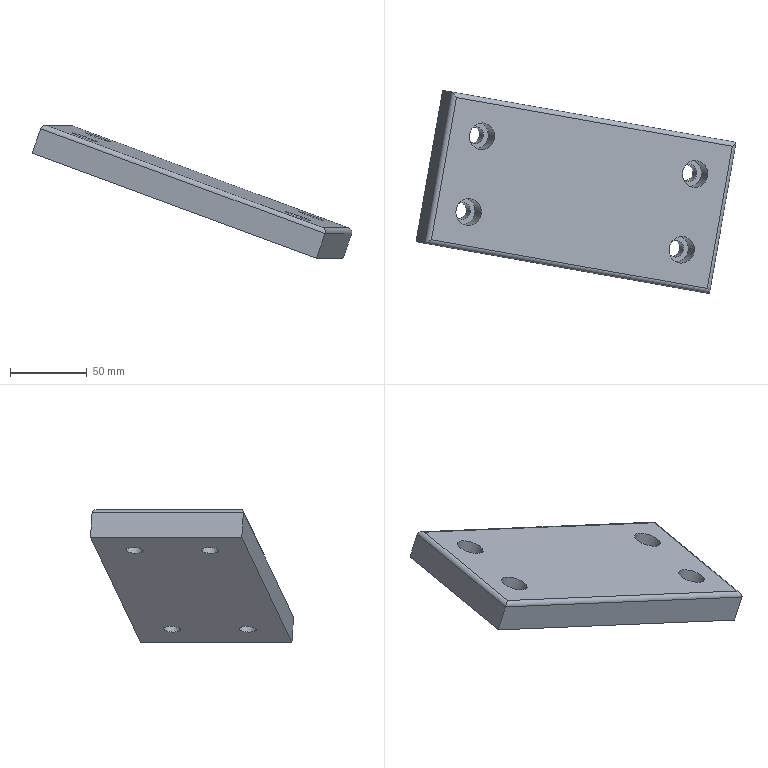Part | NX | features solid 2 | 1 solid | 22 faces | box 208.326 x 132.13 x 86.353 mm | volume 384265 mm3 | cylinder 12 | plane 10 | commonest cylinder face diameters 6 x4 11 x4 17.5 x4
STEP:
#1=CARTESIAN_POINT('',(-905.367,162.289,-231.832));
#2=VERTEX_POINT('',#1);
#3=CARTESIAN_POINT('',(-1090.45,194.924,-163.428));
#4=VERTEX_POINT('',#3);
#5=CARTESIAN_POINT('',(-905.275,162.273,-231.866));
#6=DIRECTION('',(-0.9254,0.1632,0.342));
#7=VECTOR('',#6,1000.);
#8=LINE('',#5,#7);
#9=EDGE_CURVE('',#2,#4,#8,.T.);
#10=ORIENTED_EDGE('',*,*,#9,.T.);
#11=CARTESIAN_POINT('',(-1096.176,195.934,-179.402));
#12=VERTEX_POINT('',#11);
#13=CARTESIAN_POINT('',(-1089.406,194.74,-160.515));
#14=DIRECTION('',(-0.3368,0.05939,-0.9397));
#15=VECTOR('',#14,1000.);
#16=LINE('',#13,#15);
#17=EDGE_CURVE('',#4,#12,#16,.T.);
#18=ORIENTED_EDGE('',*,*,#17,.T.);
#19=CARTESIAN_POINT('',(-911.093,163.299,-247.806));
#20=VERTEX_POINT('',#19);
#21=CARTESIAN_POINT('',(-910.908,163.266,-247.875));
#22=DIRECTION('',(-0.9254,0.1632,0.342));
#23=VECTOR('',#22,1000.);
#24=LINE('',#21,#23);
#25=EDGE_CURVE('',#20,#12,#24,.T.);
#26=ORIENTED_EDGE('',*,*,#25,.F.);
#27=CARTESIAN_POINT('',(-911.464,163.364,-248.84));
#28=DIRECTION('',(0.3368,-0.05939,0.9397));
#29=VECTOR('',#28,1000.);
#30=LINE('',#27,#29);
#31=EDGE_CURVE('',#2,#20,#30,.F.);
#32=ORIENTED_EDGE('',*,*,#31,.F.);
#33=EDGE_LOOP('',(#10,#18,#26,#32));
#34=FACE_BOUND('',#33,.T.);
#35=CARTESIAN_POINT('',(-904.23,162.089,-228.953));
#36=DIRECTION('',(-0.1736,-0.9848,0.));
#37=DIRECTION('',(-0.9254,0.1632,0.342));
#38=AXIS2_PLACEMENT_3D('',#35,#36,#37);
#39=PLANE('',#38);
#40=ADVANCED_FACE('',(#34),#39,.T.);
#41=CARTESIAN_POINT('',(-906.612,165.555,-227.987));
#42=VERTEX_POINT('',#41);
#43=CARTESIAN_POINT('',(-907.622,165.733,-230.806));
#44=DIRECTION('',(0.7772,0.581,-0.2418));
#45=DIRECTION('',(-0.5316,0.8117,0.2418));
#46=AXIS2_PLACEMENT_3D('',#43,#44,#45);
#47=ELLIPSE('',#46,4.243,3.);
#48=EDGE_CURVE('',#42,#2,#47,.T.);
#49=ORIENTED_EDGE('',*,*,#48,.T.);
#50=CARTESIAN_POINT('',(-888.002,260.77,-231.832));
#51=VERTEX_POINT('',#50);
#52=CARTESIAN_POINT('',(-906.053,158.399,-231.832));
#53=DIRECTION('',(0.1736,0.9848,0.));
#54=VECTOR('',#53,1000.);
#55=LINE('',#52,#54);
#56=EDGE_CURVE('',#51,#2,#55,.F.);
#57=ORIENTED_EDGE('',*,*,#56,.F.);
#58=CARTESIAN_POINT('',(-890.289,258.127,-227.987));
#59=VERTEX_POINT('',#58);
#60=CARTESIAN_POINT('',(-891.3,258.305,-230.806));
#61=DIRECTION('',(-0.5316,0.8117,0.2418));
#62=DIRECTION('',(0.7772,0.581,-0.2418));
#63=AXIS2_PLACEMENT_3D('',#60,#61,#62);
#64=ELLIPSE('',#63,4.243,3.);
#65=EDGE_CURVE('',#59,#51,#64,.T.);
#66=ORIENTED_EDGE('',*,*,#65,.F.);
#67=CARTESIAN_POINT('',(-887.58,273.49,-227.987));
#68=DIRECTION('',(0.1736,0.9848,0.));
#69=VECTOR('',#68,1000.);
#70=LINE('',#67,#69);
#71=EDGE_CURVE('',#42,#59,#70,.T.);
#72=ORIENTED_EDGE('',*,*,#71,.F.);
#73=EDGE_LOOP('',(#49,#57,#66,#72));
#74=FACE_BOUND('',#73,.T.);
#75=CARTESIAN_POINT('',(-888.591,273.668,-230.806));
#76=DIRECTION('',(0.1736,0.9848,0.));
#77=DIRECTION('',(-0.9848,0.1736,0.));
#78=AXIS2_PLACEMENT_3D('',#75,#76,#77);
#79=CYLINDRICAL_SURFACE('',#78,3.);
#80=ADVANCED_FACE('',(#74),#79,.T.);
#81=CARTESIAN_POINT('',(-1086.143,197.211,-161.635));
#82=VERTEX_POINT('',#81);
#83=CARTESIAN_POINT('',(-903.651,165.033,-229.081));
#84=DIRECTION('',(-0.9254,0.1632,0.342));
#85=VECTOR('',#84,1000.);
#86=LINE('',#83,#85);
#87=EDGE_CURVE('',#82,#42,#86,.F.);
#88=ORIENTED_EDGE('',*,*,#87,.F.);
#89=CARTESIAN_POINT('',(-1087.153,197.389,-164.454));
#90=DIRECTION('',(-0.5316,0.8117,0.2418));
#91=DIRECTION('',(-0.7772,-0.581,0.2418));
#92=AXIS2_PLACEMENT_3D('',#89,#90,#91);
#93=ELLIPSE('',#92,4.243,3.);
#94=EDGE_CURVE('',#4,#82,#93,.T.);
#95=ORIENTED_EDGE('',*,*,#94,.F.);
#96=ORIENTED_EDGE('',*,*,#9,.F.);
#97=ORIENTED_EDGE('',*,*,#48,.F.);
#98=EDGE_LOOP('',(#88,#95,#96,#97));
#99=FACE_BOUND('',#98,.T.);
#100=CARTESIAN_POINT('',(-904.754,165.227,-231.866));
#101=DIRECTION('',(-0.9254,0.1632,0.342));
#102=DIRECTION('',(0.3368,-0.05939,0.9397));
#103=AXIS2_PLACEMENT_3D('',#100,#101,#102);
#104=CYLINDRICAL_SURFACE('',#103,3.);
#105=ADVANCED_FACE('',(#99),#104,.T.);
#106=ORIENTED_EDGE('',*,*,#71,.T.);
#107=CARTESIAN_POINT('',(-1069.82,289.783,-161.635));
#108=VERTEX_POINT('',#107);
#109=CARTESIAN_POINT('',(-887.328,257.605,-229.081));
#110=DIRECTION('',(-0.9254,0.1632,0.342));
#111=VECTOR('',#110,1000.);
#112=LINE('',#109,#111);
#113=EDGE_CURVE('',#59,#108,#112,.T.);
#114=ORIENTED_EDGE('',*,*,#113,.T.);
#115=CARTESIAN_POINT('',(-1067.111,305.146,-161.635));
#116=DIRECTION('',(0.1736,0.9848,0.));
#117=VECTOR('',#116,1000.);
#118=LINE('',#115,#117);
#119=EDGE_CURVE('',#108,#82,#118,.F.);
#120=ORIENTED_EDGE('',*,*,#119,.T.);
#121=ORIENTED_EDGE('',*,*,#87,.T.);
#122=EDGE_LOOP('',(#106,#114,#120,#121));
#123=FACE_BOUND('',#122,.T.);
#124=CARTESIAN_POINT('',(-922.566,241.479,-217.469));
#125=VERTEX_POINT('',#124);
#126=CARTESIAN_POINT('',(-914.468,240.051,-220.462));
#127=DIRECTION('',(-0.3368,0.05939,-0.9397));
#128=DIRECTION('',(-0.9254,0.1632,0.342));
#129=AXIS2_PLACEMENT_3D('',#126,#127,#128);
#130=CIRCLE('',#129,8.75);
#131=EDGE_CURVE('',#125,#125,#130,.T.);
#132=ORIENTED_EDGE('',*,*,#131,.T.);
#133=EDGE_LOOP('',(#132));
#134=FACE_BOUND('',#133,.T.);
#135=CARTESIAN_POINT('',(-931.248,192.238,-217.469));
#136=VERTEX_POINT('',#135);
#137=CARTESIAN_POINT('',(-923.151,190.811,-220.462));
#138=DIRECTION('',(-0.3368,0.05939,-0.9397));
#139=DIRECTION('',(-0.9254,0.1632,0.342));
#140=AXIS2_PLACEMENT_3D('',#137,#138,#139);
#141=CIRCLE('',#140,8.75);
#142=EDGE_CURVE('',#136,#136,#141,.T.);
#143=ORIENTED_EDGE('',*,*,#142,.T.);
#144=EDGE_LOOP('',(#143));
#145=FACE_BOUND('',#144,.T.);
#146=CARTESIAN_POINT('',(-1053.866,213.859,-172.152));
#147=VERTEX_POINT('',#146);
#148=CARTESIAN_POINT('',(-1061.963,215.287,-169.159));
#149=DIRECTION('',(0.3368,-0.05939,0.9397));
#150=DIRECTION('',(0.9254,-0.1632,-0.342));
#151=AXIS2_PLACEMENT_3D('',#148,#149,#150);
#152=CIRCLE('',#151,8.75);
#153=EDGE_CURVE('',#147,#147,#152,.F.);
#154=ORIENTED_EDGE('',*,*,#153,.T.);
#155=EDGE_LOOP('',(#154));
#156=FACE_BOUND('',#155,.T.);
#157=CARTESIAN_POINT('',(-1045.184,263.1,-172.152));
#158=VERTEX_POINT('',#157);
#159=CARTESIAN_POINT('',(-1053.281,264.527,-169.159));
#160=DIRECTION('',(0.3368,-0.05939,0.9397));
#161=DIRECTION('',(0.9254,-0.1632,-0.342));
#162=AXIS2_PLACEMENT_3D('',#159,#160,#161);
#163=CIRCLE('',#162,8.75);
#164=EDGE_CURVE('',#158,#158,#163,.F.);
#165=ORIENTED_EDGE('',*,*,#164,.T.);
#166=EDGE_LOOP('',(#165));
#167=FACE_BOUND('',#166,.T.);
#168=CARTESIAN_POINT('',(-884.619,272.968,-229.081));
#169=DIRECTION('',(0.3368,-0.05939,0.9397));
#170=DIRECTION('',(-0.9254,0.1632,0.342));
#171=AXIS2_PLACEMENT_3D('',#168,#169,#170);
#172=PLANE('',#171);
#173=ADVANCED_FACE('',(#123,#134,#145,#156,#167),#172,.T.);
#174=ORIENTED_EDGE('',*,*,#31,.T.);
#175=CARTESIAN_POINT('',(-893.728,261.78,-247.806));
#176=VERTEX_POINT('',#175);
#177=CARTESIAN_POINT('',(-891.558,274.09,-247.806));
#178=DIRECTION('',(-0.1736,-0.9848,0.));
#179=VECTOR('',#178,1000.);
#180=LINE('',#177,#179);
#181=EDGE_CURVE('',#176,#20,#180,.T.);
#182=ORIENTED_EDGE('',*,*,#181,.F.);
#183=CARTESIAN_POINT('',(-894.099,261.845,-248.84));
#184=DIRECTION('',(0.3368,-0.05939,0.9397));
#185=VECTOR('',#184,1000.);
#186=LINE('',#183,#185);
#187=EDGE_CURVE('',#176,#51,#186,.T.);
#188=ORIENTED_EDGE('',*,*,#187,.T.);
#189=ORIENTED_EDGE('',*,*,#56,.T.);
#190=EDGE_LOOP('',(#174,#182,#188,#189));
#191=FACE_BOUND('',#190,.T.);
#192=CARTESIAN_POINT('',(-912.15,159.474,-248.84));
#193=DIRECTION('',(0.9254,-0.1632,-0.342));
#194=DIRECTION('',(0.1736,0.9848,0.));
#195=AXIS2_PLACEMENT_3D('',#192,#193,#194);
#196=PLANE('',#195);
#197=ADVANCED_FACE('',(#191),#196,.T.);
#198=ORIENTED_EDGE('',*,*,#25,.T.);
#199=CARTESIAN_POINT('',(-1078.812,294.415,-179.402));
#200=VERTEX_POINT('',#199);
#201=CARTESIAN_POINT('',(-1093.85,209.13,-179.402));
#202=DIRECTION('',(-0.1736,-0.9848,0.));
#203=VECTOR('',#202,1000.);
#204=LINE('',#201,#203);
#205=EDGE_CURVE('',#200,#12,#204,.T.);
#206=ORIENTED_EDGE('',*,*,#205,.F.);
#207=CARTESIAN_POINT('',(-893.543,261.747,-247.875));
#208=DIRECTION('',(0.9254,-0.1632,-0.342));
#209=VECTOR('',#208,1000.);
#210=LINE('',#207,#209);
#211=EDGE_CURVE('',#200,#176,#210,.T.);
#212=ORIENTED_EDGE('',*,*,#211,.T.);
#213=ORIENTED_EDGE('',*,*,#181,.T.);
#214=EDGE_LOOP('',(#198,#206,#212,#213));
#215=FACE_BOUND('',#214,.T.);
#216=CARTESIAN_POINT('',(-926.295,242.136,-237.375));
#217=VERTEX_POINT('',#216);
#218=CARTESIAN_POINT('',(-921.205,241.239,-239.256));
#219=DIRECTION('',(-0.3368,0.05939,-0.9397));
#220=DIRECTION('',(-0.9254,0.1632,0.342));
#221=AXIS2_PLACEMENT_3D('',#218,#219,#220);
#222=CIRCLE('',#221,5.5);
#223=EDGE_CURVE('',#217,#217,#222,.T.);
#224=ORIENTED_EDGE('',*,*,#223,.F.);
#225=EDGE_LOOP('',(#224));
#226=FACE_BOUND('',#225,.T.);
#227=CARTESIAN_POINT('',(-934.977,192.896,-237.375));
#228=VERTEX_POINT('',#227);
#229=CARTESIAN_POINT('',(-929.887,191.998,-239.256));
#230=DIRECTION('',(-0.3368,0.05939,-0.9397));
#231=DIRECTION('',(-0.9254,0.1632,0.342));
#232=AXIS2_PLACEMENT_3D('',#229,#230,#231);
#233=CIRCLE('',#232,5.5);
#234=EDGE_CURVE('',#228,#228,#233,.T.);
#235=ORIENTED_EDGE('',*,*,#234,.F.);
#236=EDGE_LOOP('',(#235));
#237=FACE_BOUND('',#236,.T.);
#238=CARTESIAN_POINT('',(-1073.79,217.372,-186.072));
#239=VERTEX_POINT('',#238);
#240=CARTESIAN_POINT('',(-1068.7,216.475,-187.953));
#241=DIRECTION('',(-0.3368,0.05939,-0.9397));
#242=DIRECTION('',(-0.9254,0.1632,0.342));
#243=AXIS2_PLACEMENT_3D('',#240,#241,#242);
#244=CIRCLE('',#243,5.5);
#245=EDGE_CURVE('',#239,#239,#244,.T.);
#246=ORIENTED_EDGE('',*,*,#245,.F.);
#247=EDGE_LOOP('',(#246));
#248=FACE_BOUND('',#247,.T.);
#249=CARTESIAN_POINT('',(-1065.107,266.613,-186.072));
#250=VERTEX_POINT('',#249);
#251=CARTESIAN_POINT('',(-1060.017,265.715,-187.953));
#252=DIRECTION('',(-0.3368,0.05939,-0.9397));
#253=DIRECTION('',(-0.9254,0.1632,0.342));
#254=AXIS2_PLACEMENT_3D('',#251,#252,#253);
#255=CIRCLE('',#254,5.5);
#256=EDGE_CURVE('',#250,#250,#255,.T.);
#257=ORIENTED_EDGE('',*,*,#256,.F.);
#258=EDGE_LOOP('',(#257));
#259=FACE_BOUND('',#258,.T.);
#260=CARTESIAN_POINT('',(-911.611,159.278,-247.875));
#261=DIRECTION('',(-0.3368,0.05939,-0.9397));
#262=DIRECTION('',(-0.9254,0.1632,0.342));
#263=AXIS2_PLACEMENT_3D('',#260,#261,#262);
#264=PLANE('',#263);
#265=ADVANCED_FACE('',(#215,#226,#237,#248,#259),#264,.T.);
#266=ORIENTED_EDGE('',*,*,#17,.F.);
#267=CARTESIAN_POINT('',(-1073.086,293.405,-163.428));
#268=VERTEX_POINT('',#267);
#269=CARTESIAN_POINT('',(-1088.124,208.121,-163.428));
#270=DIRECTION('',(0.1736,0.9848,0.));
#271=VECTOR('',#270,1000.);
#272=LINE('',#269,#271);
#273=EDGE_CURVE('',#4,#268,#272,.T.);
#274=ORIENTED_EDGE('',*,*,#273,.T.);
#275=CARTESIAN_POINT('',(-1072.041,293.221,-160.515));
#276=DIRECTION('',(-0.3368,0.05939,-0.9397));
#277=VECTOR('',#276,1000.);
#278=LINE('',#275,#277);
#279=EDGE_CURVE('',#268,#200,#278,.T.);
#280=ORIENTED_EDGE('',*,*,#279,.T.);
#281=ORIENTED_EDGE('',*,*,#205,.T.);
#282=EDGE_LOOP('',(#266,#274,#280,#281));
#283=FACE_BOUND('',#282,.T.);
#284=CARTESIAN_POINT('',(-1087.079,207.937,-160.515));
#285=DIRECTION('',(-0.9254,0.1632,0.342));
#286=DIRECTION('',(0.1736,0.9848,0.));
#287=AXIS2_PLACEMENT_3D('',#284,#285,#286);
#288=PLANE('',#287);
#289=ADVANCED_FACE('',(#283),#288,.T.);
#290=ORIENTED_EDGE('',*,*,#279,.F.);
#291=CARTESIAN_POINT('',(-881.062,259.546,-234.397));
#292=DIRECTION('',(-0.9254,0.1632,0.342));
#293=VECTOR('',#292,1000.);
#294=LINE('',#291,#293);
#295=EDGE_CURVE('',#268,#51,#294,.F.);
#296=ORIENTED_EDGE('',*,*,#295,.T.);
#297=ORIENTED_EDGE('',*,*,#187,.F.);
#298=ORIENTED_EDGE('',*,*,#211,.F.);
#299=EDGE_LOOP('',(#290,#296,#297,#298));
#300=FACE_BOUND('',#299,.T.);
#301=CARTESIAN_POINT('',(-887.125,260.615,-251.311));
#302=DIRECTION('',(0.1736,0.9848,0.));
#303=DIRECTION('',(-0.9254,0.1632,0.342));
#304=AXIS2_PLACEMENT_3D('',#301,#302,#303);
#305=PLANE('',#304);
#306=ADVANCED_FACE('',(#300),#305,.T.);
#307=ORIENTED_EDGE('',*,*,#223,.T.);
#308=EDGE_LOOP('',(#307));
#309=FACE_BOUND('',#308,.T.);
#310=CARTESIAN_POINT('',(-923.6,241.661,-229.857));
#311=VERTEX_POINT('',#310);
#312=CARTESIAN_POINT('',(-918.51,240.764,-231.738));
#313=DIRECTION('',(-0.3368,0.05939,-0.9397));
#314=DIRECTION('',(-0.9254,0.1632,0.342));
#315=AXIS2_PLACEMENT_3D('',#312,#313,#314);
#316=CIRCLE('',#315,5.5);
#317=EDGE_CURVE('',#311,#311,#316,.T.);
#318=ORIENTED_EDGE('',*,*,#317,.F.);
#319=EDGE_LOOP('',(#318));
#320=FACE_BOUND('',#319,.T.);
#321=CARTESIAN_POINT('',(-931.31,243.021,-267.447));
#322=DIRECTION('',(-0.3368,0.05939,-0.9397));
#323=DIRECTION('',(-0.9254,0.1632,0.342));
#324=AXIS2_PLACEMENT_3D('',#321,#322,#323);
#325=CYLINDRICAL_SURFACE('',#324,5.5);
#326=ADVANCED_FACE('',(#309,#320),#325,.F.);
#327=ORIENTED_EDGE('',*,*,#317,.T.);
#328=EDGE_LOOP('',(#327));
#329=FACE_BOUND('',#328,.T.);
#330=CARTESIAN_POINT('',(-926.608,242.191,-228.746));
#331=VERTEX_POINT('',#330);
#332=CARTESIAN_POINT('',(-918.51,240.764,-231.738));
#333=DIRECTION('',(-0.3368,0.05939,-0.9397));
#334=DIRECTION('',(-0.9254,0.1632,0.342));
#335=AXIS2_PLACEMENT_3D('',#332,#333,#334);
#336=CIRCLE('',#335,8.75);
#337=EDGE_CURVE('',#331,#331,#336,.T.);
#338=ORIENTED_EDGE('',*,*,#337,.F.);
#339=EDGE_LOOP('',(#338));
#340=FACE_BOUND('',#339,.T.);
#341=CARTESIAN_POINT('',(-920.594,228.946,-231.738));
#342=DIRECTION('',(-0.3368,0.05939,-0.9397));
#343=DIRECTION('',(-0.9254,0.1632,0.342));
#344=AXIS2_PLACEMENT_3D('',#341,#342,#343);
#345=PLANE('',#344);
#346=ADVANCED_FACE('',(#329,#340),#345,.F.);
#347=ORIENTED_EDGE('',*,*,#337,.T.);
#348=EDGE_LOOP('',(#347));
#349=FACE_BOUND('',#348,.T.);
#350=ORIENTED_EDGE('',*,*,#131,.F.);
#351=EDGE_LOOP('',(#350));
#352=FACE_BOUND('',#351,.T.);
#353=CARTESIAN_POINT('',(-914.468,240.051,-220.462));
#354=DIRECTION('',(-0.3368,0.05939,-0.9397));
#355=DIRECTION('',(-0.9254,0.1632,0.342));
#356=AXIS2_PLACEMENT_3D('',#353,#354,#355);
#357=CYLINDRICAL_SURFACE('',#356,8.75);
#358=ADVANCED_FACE('',(#349,#352),#357,.F.);
#359=ORIENTED_EDGE('',*,*,#234,.T.);
#360=EDGE_LOOP('',(#359));
#361=FACE_BOUND('',#360,.T.);
#362=CARTESIAN_POINT('',(-932.283,192.421,-229.857));
#363=VERTEX_POINT('',#362);
#364=CARTESIAN_POINT('',(-927.193,191.523,-231.738));
#365=DIRECTION('',(-0.3368,0.05939,-0.9397));
#366=DIRECTION('',(-0.9254,0.1632,0.342));
#367=AXIS2_PLACEMENT_3D('',#364,#365,#366);
#368=CIRCLE('',#367,5.5);
#369=EDGE_CURVE('',#363,#363,#368,.T.);
#370=ORIENTED_EDGE('',*,*,#369,.F.);
#371=EDGE_LOOP('',(#370));
#372=FACE_BOUND('',#371,.T.);
#373=CARTESIAN_POINT('',(-939.992,193.78,-267.447));
#374=DIRECTION('',(-0.3368,0.05939,-0.9397));
#375=DIRECTION('',(-0.9254,0.1632,0.342));
#376=AXIS2_PLACEMENT_3D('',#373,#374,#375);
#377=CYLINDRICAL_SURFACE('',#376,5.5);
#378=ADVANCED_FACE('',(#361,#372),#377,.F.);
#379=ORIENTED_EDGE('',*,*,#369,.T.);
#380=EDGE_LOOP('',(#379));
#381=FACE_BOUND('',#380,.T.);
#382=CARTESIAN_POINT('',(-935.29,192.951,-228.746));
#383=VERTEX_POINT('',#382);
#384=CARTESIAN_POINT('',(-927.193,191.523,-231.738));
#385=DIRECTION('',(-0.3368,0.05939,-0.9397));
#386=DIRECTION('',(-0.9254,0.1632,0.342));
#387=AXIS2_PLACEMENT_3D('',#384,#385,#386);
#388=CIRCLE('',#387,8.75);
#389=EDGE_CURVE('',#383,#383,#388,.T.);
#390=ORIENTED_EDGE('',*,*,#389,.F.);
#391=EDGE_LOOP('',(#390));
#392=FACE_BOUND('',#391,.T.);
#393=CARTESIAN_POINT('',(-924.935,204.326,-231.738));
#394=DIRECTION('',(-0.3368,0.05939,-0.9397));
#395=DIRECTION('',(-0.9254,0.1632,0.342));
#396=AXIS2_PLACEMENT_3D('',#393,#394,#395);
#397=PLANE('',#396);
#398=ADVANCED_FACE('',(#381,#392),#397,.F.);
#399=ORIENTED_EDGE('',*,*,#389,.T.);
#400=EDGE_LOOP('',(#399));
#401=FACE_BOUND('',#400,.T.);
#402=ORIENTED_EDGE('',*,*,#142,.F.);
#403=EDGE_LOOP('',(#402));
#404=FACE_BOUND('',#403,.T.);
#405=CARTESIAN_POINT('',(-923.151,190.811,-220.462));
#406=DIRECTION('',(-0.3368,0.05939,-0.9397));
#407=DIRECTION('',(-0.9254,0.1632,0.342));
#408=AXIS2_PLACEMENT_3D('',#405,#406,#407);
#409=CYLINDRICAL_SURFACE('',#408,8.75);
#410=ADVANCED_FACE('',(#401,#404),#409,.F.);
#411=ORIENTED_EDGE('',*,*,#245,.T.);
#412=EDGE_LOOP('',(#411));
#413=FACE_BOUND('',#412,.T.);
#414=CARTESIAN_POINT('',(-1071.095,216.897,-178.554));
#415=VERTEX_POINT('',#414);
#416=CARTESIAN_POINT('',(-1066.005,216.,-180.435));
#417=DIRECTION('',(-0.3368,0.05939,-0.9397));
#418=DIRECTION('',(-0.9254,0.1632,0.342));
#419=AXIS2_PLACEMENT_3D('',#416,#417,#418);
#420=CIRCLE('',#419,5.5);
#421=EDGE_CURVE('',#415,#415,#420,.T.);
#422=ORIENTED_EDGE('',*,*,#421,.F.);
#423=EDGE_LOOP('',(#422));
#424=FACE_BOUND('',#423,.T.);
#425=CARTESIAN_POINT('',(-1078.805,218.257,-216.144));
#426=DIRECTION('',(-0.3368,0.05939,-0.9397));
#427=DIRECTION('',(-0.9254,0.1632,0.342));
#428=AXIS2_PLACEMENT_3D('',#425,#426,#427);
#429=CYLINDRICAL_SURFACE('',#428,5.5);
#430=ADVANCED_FACE('',(#413,#424),#429,.F.);
#431=ORIENTED_EDGE('',*,*,#421,.T.);
#432=EDGE_LOOP('',(#431));
#433=FACE_BOUND('',#432,.T.);
#434=CARTESIAN_POINT('',(-1074.103,217.427,-177.443));
#435=VERTEX_POINT('',#434);
#436=CARTESIAN_POINT('',(-1066.005,216.,-180.435));
#437=DIRECTION('',(-0.3368,0.05939,-0.9397));
#438=DIRECTION('',(-0.9254,0.1632,0.342));
#439=AXIS2_PLACEMENT_3D('',#436,#437,#438);
#440=CIRCLE('',#439,8.75);
#441=EDGE_CURVE('',#435,#435,#440,.T.);
#442=ORIENTED_EDGE('',*,*,#441,.F.);
#443=EDGE_LOOP('',(#442));
#444=FACE_BOUND('',#443,.T.);
#445=CARTESIAN_POINT('',(-1110.019,236.961,-163.334));
#446=DIRECTION('',(-0.3368,0.05939,-0.9397));
#447=DIRECTION('',(-0.9254,0.1632,0.342));
#448=AXIS2_PLACEMENT_3D('',#445,#446,#447);
#449=PLANE('',#448);
#450=ADVANCED_FACE('',(#433,#444),#449,.F.);
#451=ORIENTED_EDGE('',*,*,#441,.T.);
#452=EDGE_LOOP('',(#451));
#453=FACE_BOUND('',#452,.T.);
#454=ORIENTED_EDGE('',*,*,#153,.F.);
#455=EDGE_LOOP('',(#454));
#456=FACE_BOUND('',#455,.T.);
#457=CARTESIAN_POINT('',(-1061.963,215.287,-169.159));
#458=DIRECTION('',(-0.3368,0.05939,-0.9397));
#459=DIRECTION('',(-0.9254,0.1632,0.342));
#460=AXIS2_PLACEMENT_3D('',#457,#458,#459);
#461=CYLINDRICAL_SURFACE('',#460,8.75);
#462=ADVANCED_FACE('',(#453,#456),#461,.F.);
#463=ORIENTED_EDGE('',*,*,#256,.T.);
#464=EDGE_LOOP('',(#463));
#465=FACE_BOUND('',#464,.T.);
#466=CARTESIAN_POINT('',(-1062.413,266.138,-178.554));
#467=VERTEX_POINT('',#466);
#468=CARTESIAN_POINT('',(-1057.323,265.24,-180.435));
#469=DIRECTION('',(-0.3368,0.05939,-0.9397));
#470=DIRECTION('',(-0.9254,0.1632,0.342));
#471=AXIS2_PLACEMENT_3D('',#468,#469,#470);
#472=CIRCLE('',#471,5.5);
#473=EDGE_CURVE('',#467,#467,#472,.T.);
#474=ORIENTED_EDGE('',*,*,#473,.F.);
#475=EDGE_LOOP('',(#474));
#476=FACE_BOUND('',#475,.T.);
#477=CARTESIAN_POINT('',(-1070.122,267.497,-216.144));
#478=DIRECTION('',(-0.3368,0.05939,-0.9397));
#479=DIRECTION('',(-0.9254,0.1632,0.342));
#480=AXIS2_PLACEMENT_3D('',#477,#478,#479);
#481=CYLINDRICAL_SURFACE('',#480,5.5);
#482=ADVANCED_FACE('',(#465,#476),#481,.F.);
#483=ORIENTED_EDGE('',*,*,#473,.T.);
#484=EDGE_LOOP('',(#483));
#485=FACE_BOUND('',#484,.T.);
#486=CARTESIAN_POINT('',(-1065.42,266.668,-177.443));
#487=VERTEX_POINT('',#486);
#488=CARTESIAN_POINT('',(-1057.323,265.24,-180.435));
#489=DIRECTION('',(-0.3368,0.05939,-0.9397));
#490=DIRECTION('',(-0.9254,0.1632,0.342));
#491=AXIS2_PLACEMENT_3D('',#488,#489,#490);
#492=CIRCLE('',#491,8.75);
#493=EDGE_CURVE('',#487,#487,#492,.T.);
#494=ORIENTED_EDGE('',*,*,#493,.F.);
#495=EDGE_LOOP('',(#494));
#496=FACE_BOUND('',#495,.T.);
#497=CARTESIAN_POINT('',(-1059.407,253.422,-180.435));
#498=DIRECTION('',(-0.3368,0.05939,-0.9397));
#499=DIRECTION('',(-0.9254,0.1632,0.342));
#500=AXIS2_PLACEMENT_3D('',#497,#498,#499);
#501=PLANE('',#500);
#502=ADVANCED_FACE('',(#485,#496),#501,.F.);
#503=ORIENTED_EDGE('',*,*,#493,.T.);
#504=EDGE_LOOP('',(#503));
#505=FACE_BOUND('',#504,.T.);
#506=ORIENTED_EDGE('',*,*,#164,.F.);
#507=EDGE_LOOP('',(#506));
#508=FACE_BOUND('',#507,.T.);
#509=CARTESIAN_POINT('',(-1053.281,264.527,-169.159));
#510=DIRECTION('',(-0.3368,0.05939,-0.9397));
#511=DIRECTION('',(-0.9254,0.1632,0.342));
#512=AXIS2_PLACEMENT_3D('',#509,#510,#511);
#513=CYLINDRICAL_SURFACE('',#512,8.75);
#514=ADVANCED_FACE('',(#505,#508),#513,.F.);
#515=ORIENTED_EDGE('',*,*,#65,.T.);
#516=ORIENTED_EDGE('',*,*,#295,.F.);
#517=CARTESIAN_POINT('',(-1070.83,289.961,-164.454));
#518=DIRECTION('',(-0.7772,-0.581,0.2418));
#519=DIRECTION('',(-0.5316,0.8117,0.2418));
#520=AXIS2_PLACEMENT_3D('',#517,#518,#519);
#521=ELLIPSE('',#520,4.243,3.);
#522=EDGE_CURVE('',#108,#268,#521,.T.);
#523=ORIENTED_EDGE('',*,*,#522,.F.);
#524=ORIENTED_EDGE('',*,*,#113,.F.);
#525=EDGE_LOOP('',(#515,#516,#523,#524));
#526=FACE_BOUND('',#525,.T.);
#527=CARTESIAN_POINT('',(-888.338,257.783,-231.9));
#528=DIRECTION('',(-0.9254,0.1632,0.342));
#529=DIRECTION('',(0.3368,-0.05939,0.9397));
#530=AXIS2_PLACEMENT_3D('',#527,#528,#529);
#531=CYLINDRICAL_SURFACE('',#530,3.);
#532=ADVANCED_FACE('',(#526),#531,.T.);
#533=ORIENTED_EDGE('',*,*,#94,.T.);
#534=ORIENTED_EDGE('',*,*,#119,.F.);
#535=ORIENTED_EDGE('',*,*,#522,.T.);
#536=ORIENTED_EDGE('',*,*,#273,.F.);
#537=EDGE_LOOP('',(#533,#534,#535,#536));
#538=FACE_BOUND('',#537,.T.);
#539=CARTESIAN_POINT('',(-1085.347,207.631,-164.454));
#540=DIRECTION('',(0.1736,0.9848,0.));
#541=DIRECTION('',(-0.9848,0.1736,0.));
#542=AXIS2_PLACEMENT_3D('',#539,#540,#541);
#543=CYLINDRICAL_SURFACE('',#542,3.);
#544=ADVANCED_FACE('',(#538),#543,.T.);
#545=CLOSED_SHELL('',(#40,#80,#105,#173,#197,#265,#289,#306,#326,#346,#358,#378,#398,#410,#430,#450,#462,#482,#502,#514,#532,#544));
#546=MANIFOLD_SOLID_BREP('',#545);
#547=(LENGTH_UNIT()NAMED_UNIT(*)SI_UNIT(.MILLI.,.METRE.));
#548=UNCERTAINTY_MEASURE_WITH_UNIT(LENGTH_MEASURE(0.00001),#547,'','');
#549=(NAMED_UNIT(*)PLANE_ANGLE_UNIT()SI_UNIT($,.RADIAN.));
#550=(NAMED_UNIT(*)SI_UNIT($,.STERADIAN.)SOLID_ANGLE_UNIT());
#551=(GEOMETRIC_REPRESENTATION_CONTEXT(3)GLOBAL_UNCERTAINTY_ASSIGNED_CONTEXT((#548))GLOBAL_UNIT_ASSIGNED_CONTEXT((#547,#549,#550))REPRESENTATION_CONTEXT('',''));
#552=ADVANCED_BREP_SHAPE_REPRESENTATION('',(#546),#551);